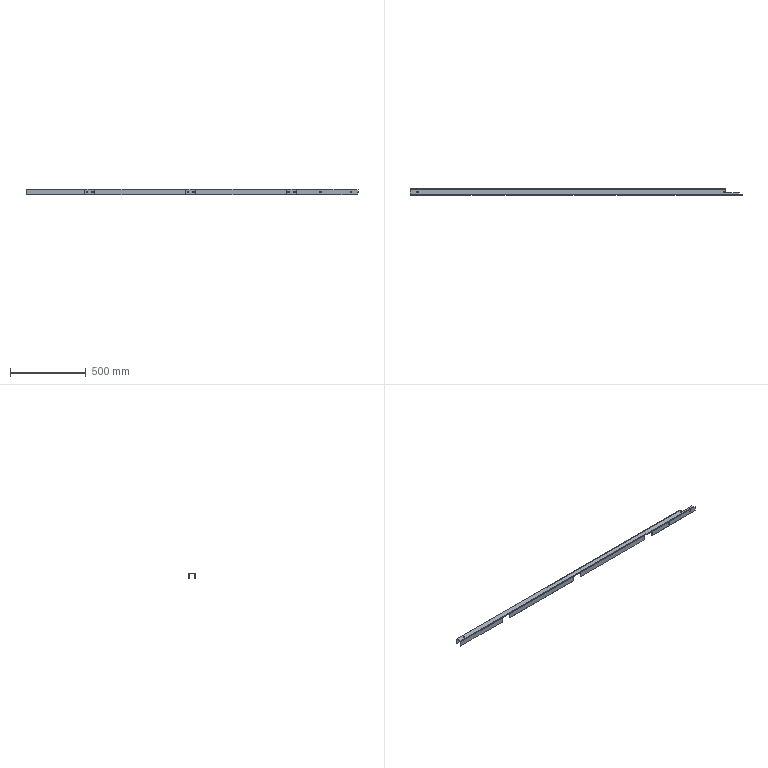Part | NX | features solid 2 | 1 solid | 101 faces | box 2198 x 40 x 38 mm | volume 452380 mm3 | plane 59 | cylinder 42 | commonest cylinder face diameters 9 x18 8.5 x12 9.2 x4 10.2 x4 4 x2 8 x2